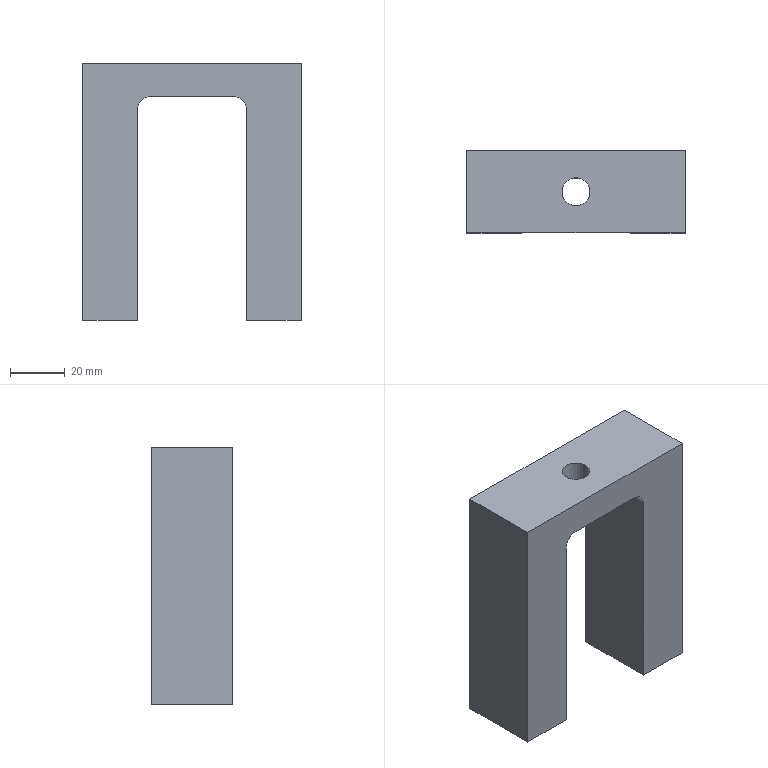Part | STEP file | 11-FG-SJ00211 | 1 solid | 38 faces | box 80 x 30 x 94 mm | volume 125576 mm3 | cylinder 16 | cone 12 | plane 10 | commonest cylinder face diameters 3.3 x8 5 x4 10 x2 10.2 x2
STEP:
#1=CARTESIAN_POINT('',(29.9,9.,70.65));
#2=VERTEX_POINT('',#1);
#3=CARTESIAN_POINT('',(29.9,9.,67.35));
#4=VERTEX_POINT('',#3);
#5=CARTESIAN_POINT('',(29.9,9.,69.));
#6=DIRECTION('',(1.,0.,0.));
#7=DIRECTION('',(0.,0.,-1.));
#8=AXIS2_PLACEMENT_3D('',#5,#6,#7);
#9=CIRCLE('',#8,1.65);
#10=EDGE_CURVE('',#2,#4,#9,.T.);
#11=ORIENTED_EDGE('',*,*,#10,.F.);
#12=CARTESIAN_POINT('',(40.,9.,70.65));
#13=VERTEX_POINT('',#12);
#14=CARTESIAN_POINT('',(40.,9.,70.65));
#15=DIRECTION('',(1.,0.,0.));
#16=VECTOR('',#15,1000.);
#17=LINE('',#14,#16);
#18=EDGE_CURVE('',#2,#13,#17,.T.);
#19=ORIENTED_EDGE('',*,*,#18,.T.);
#20=CARTESIAN_POINT('',(40.,9.,67.35));
#21=VERTEX_POINT('',#20);
#22=CARTESIAN_POINT('',(40.,9.,69.));
#23=DIRECTION('',(1.,0.,0.));
#24=DIRECTION('',(0.,0.,-1.));
#25=AXIS2_PLACEMENT_3D('',#22,#23,#24);
#26=CIRCLE('',#25,1.65);
#27=EDGE_CURVE('',#13,#21,#26,.T.);
#28=ORIENTED_EDGE('',*,*,#27,.T.);
#29=CARTESIAN_POINT('',(40.,9.,67.35));
#30=DIRECTION('',(1.,0.,0.));
#31=VECTOR('',#30,1000.);
#32=LINE('',#29,#31);
#33=EDGE_CURVE('',#4,#21,#32,.T.);
#34=ORIENTED_EDGE('',*,*,#33,.F.);
#35=EDGE_LOOP('',(#11,#19,#28,#34));
#36=FACE_OUTER_BOUND('',#35,.T.);
#37=CARTESIAN_POINT('',(40.,9.,69.));
#38=DIRECTION('',(1.,0.,0.));
#39=DIRECTION('',(0.,0.,-1.));
#40=AXIS2_PLACEMENT_3D('',#37,#38,#39);
#41=CYLINDRICAL_SURFACE('',#40,1.65);
#42=ADVANCED_FACE('',(#36),#41,.F.);
#43=CARTESIAN_POINT('',(28.909,9.,69.));
#44=VERTEX_POINT('',#43);
#45=CARTESIAN_POINT('',(29.9,9.,67.35));
#46=DIRECTION('',(0.515,0.,-0.8572));
#47=VECTOR('',#46,1000.);
#48=LINE('',#45,#47);
#49=EDGE_CURVE('',#44,#4,#48,.T.);
#50=ORIENTED_EDGE('',*,*,#49,.F.);
#51=CARTESIAN_POINT('',(29.9,9.,70.65));
#52=DIRECTION('',(0.515,0.,0.8572));
#53=VECTOR('',#52,1000.);
#54=LINE('',#51,#53);
#55=EDGE_CURVE('',#44,#2,#54,.T.);
#56=ORIENTED_EDGE('',*,*,#55,.T.);
#57=ORIENTED_EDGE('',*,*,#10,.T.);
#58=EDGE_LOOP('',(#50,#56,#57));
#59=FACE_OUTER_BOUND('',#58,.T.);
#60=CARTESIAN_POINT('',(29.9,9.,69.));
#61=DIRECTION('',(1.,0.,0.));
#62=DIRECTION('',(0.,0.,-1.));
#63=AXIS2_PLACEMENT_3D('',#60,#61,#62);
#64=CONICAL_SURFACE('',#63,1.65,1.03);
#65=ADVANCED_FACE('',(#59),#64,.F.);
#66=CARTESIAN_POINT('',(29.9,9.,86.65));
#67=VERTEX_POINT('',#66);
#68=CARTESIAN_POINT('',(29.9,9.,83.35));
#69=VERTEX_POINT('',#68);
#70=CARTESIAN_POINT('',(29.9,9.,85.));
#71=DIRECTION('',(1.,0.,0.));
#72=DIRECTION('',(0.,0.,-1.));
#73=AXIS2_PLACEMENT_3D('',#70,#71,#72);
#74=CIRCLE('',#73,1.65);
#75=EDGE_CURVE('',#67,#69,#74,.T.);
#76=ORIENTED_EDGE('',*,*,#75,.F.);
#77=CARTESIAN_POINT('',(40.,9.,86.65));
#78=VERTEX_POINT('',#77);
#79=CARTESIAN_POINT('',(40.,9.,86.65));
#80=DIRECTION('',(1.,0.,0.));
#81=VECTOR('',#80,1000.);
#82=LINE('',#79,#81);
#83=EDGE_CURVE('',#67,#78,#82,.T.);
#84=ORIENTED_EDGE('',*,*,#83,.T.);
#85=CARTESIAN_POINT('',(40.,9.,83.35));
#86=VERTEX_POINT('',#85);
#87=CARTESIAN_POINT('',(40.,9.,85.));
#88=DIRECTION('',(1.,0.,0.));
#89=DIRECTION('',(0.,0.,-1.));
#90=AXIS2_PLACEMENT_3D('',#87,#88,#89);
#91=CIRCLE('',#90,1.65);
#92=EDGE_CURVE('',#78,#86,#91,.T.);
#93=ORIENTED_EDGE('',*,*,#92,.T.);
#94=CARTESIAN_POINT('',(40.,9.,83.35));
#95=DIRECTION('',(1.,0.,0.));
#96=VECTOR('',#95,1000.);
#97=LINE('',#94,#96);
#98=EDGE_CURVE('',#69,#86,#97,.T.);
#99=ORIENTED_EDGE('',*,*,#98,.F.);
#100=EDGE_LOOP('',(#76,#84,#93,#99));
#101=FACE_OUTER_BOUND('',#100,.T.);
#102=CARTESIAN_POINT('',(40.,9.,85.));
#103=DIRECTION('',(1.,0.,0.));
#104=DIRECTION('',(0.,0.,-1.));
#105=AXIS2_PLACEMENT_3D('',#102,#103,#104);
#106=CYLINDRICAL_SURFACE('',#105,1.65);
#107=ADVANCED_FACE('',(#101),#106,.F.);
#108=CARTESIAN_POINT('',(28.909,9.,85.));
#109=VERTEX_POINT('',#108);
#110=CARTESIAN_POINT('',(29.9,9.,83.35));
#111=DIRECTION('',(0.515,0.,-0.8572));
#112=VECTOR('',#111,1000.);
#113=LINE('',#110,#112);
#114=EDGE_CURVE('',#109,#69,#113,.T.);
#115=ORIENTED_EDGE('',*,*,#114,.F.);
#116=CARTESIAN_POINT('',(29.9,9.,86.65));
#117=DIRECTION('',(0.515,0.,0.8572));
#118=VECTOR('',#117,1000.);
#119=LINE('',#116,#118);
#120=EDGE_CURVE('',#109,#67,#119,.T.);
#121=ORIENTED_EDGE('',*,*,#120,.T.);
#122=ORIENTED_EDGE('',*,*,#75,.T.);
#123=EDGE_LOOP('',(#115,#121,#122));
#124=FACE_OUTER_BOUND('',#123,.T.);
#125=CARTESIAN_POINT('',(29.9,9.,85.));
#126=DIRECTION('',(1.,0.,0.));
#127=DIRECTION('',(0.,0.,-1.));
#128=AXIS2_PLACEMENT_3D('',#125,#126,#127);
#129=CONICAL_SURFACE('',#128,1.65,1.03);
#130=ADVANCED_FACE('',(#124),#129,.F.);
#131=CARTESIAN_POINT('',(29.9,-9.,86.65));
#132=VERTEX_POINT('',#131);
#133=CARTESIAN_POINT('',(29.9,-9.,83.35));
#134=VERTEX_POINT('',#133);
#135=CARTESIAN_POINT('',(29.9,-9.,85.));
#136=DIRECTION('',(1.,0.,0.));
#137=DIRECTION('',(0.,0.,-1.));
#138=AXIS2_PLACEMENT_3D('',#135,#136,#137);
#139=CIRCLE('',#138,1.65);
#140=EDGE_CURVE('',#132,#134,#139,.T.);
#141=ORIENTED_EDGE('',*,*,#140,.F.);
#142=CARTESIAN_POINT('',(40.,-9.,86.65));
#143=VERTEX_POINT('',#142);
#144=CARTESIAN_POINT('',(40.,-9.,86.65));
#145=DIRECTION('',(1.,0.,0.));
#146=VECTOR('',#145,1000.);
#147=LINE('',#144,#146);
#148=EDGE_CURVE('',#132,#143,#147,.T.);
#149=ORIENTED_EDGE('',*,*,#148,.T.);
#150=CARTESIAN_POINT('',(40.,-9.,83.35));
#151=VERTEX_POINT('',#150);
#152=CARTESIAN_POINT('',(40.,-9.,85.));
#153=DIRECTION('',(1.,0.,0.));
#154=DIRECTION('',(0.,0.,-1.));
#155=AXIS2_PLACEMENT_3D('',#152,#153,#154);
#156=CIRCLE('',#155,1.65);
#157=EDGE_CURVE('',#143,#151,#156,.T.);
#158=ORIENTED_EDGE('',*,*,#157,.T.);
#159=CARTESIAN_POINT('',(40.,-9.,83.35));
#160=DIRECTION('',(1.,0.,0.));
#161=VECTOR('',#160,1000.);
#162=LINE('',#159,#161);
#163=EDGE_CURVE('',#134,#151,#162,.T.);
#164=ORIENTED_EDGE('',*,*,#163,.F.);
#165=EDGE_LOOP('',(#141,#149,#158,#164));
#166=FACE_OUTER_BOUND('',#165,.T.);
#167=CARTESIAN_POINT('',(40.,-9.,85.));
#168=DIRECTION('',(1.,0.,0.));
#169=DIRECTION('',(0.,0.,-1.));
#170=AXIS2_PLACEMENT_3D('',#167,#168,#169);
#171=CYLINDRICAL_SURFACE('',#170,1.65);
#172=ADVANCED_FACE('',(#166),#171,.F.);
#173=CARTESIAN_POINT('',(28.909,-9.,85.));
#174=VERTEX_POINT('',#173);
#175=CARTESIAN_POINT('',(29.9,-9.,83.35));
#176=DIRECTION('',(0.515,0.,-0.8572));
#177=VECTOR('',#176,1000.);
#178=LINE('',#175,#177);
#179=EDGE_CURVE('',#174,#134,#178,.T.);
#180=ORIENTED_EDGE('',*,*,#179,.F.);
#181=CARTESIAN_POINT('',(29.9,-9.,86.65));
#182=DIRECTION('',(0.515,0.,0.8572));
#183=VECTOR('',#182,1000.);
#184=LINE('',#181,#183);
#185=EDGE_CURVE('',#174,#132,#184,.T.);
#186=ORIENTED_EDGE('',*,*,#185,.T.);
#187=ORIENTED_EDGE('',*,*,#140,.T.);
#188=EDGE_LOOP('',(#180,#186,#187));
#189=FACE_OUTER_BOUND('',#188,.T.);
#190=CARTESIAN_POINT('',(29.9,-9.,85.));
#191=DIRECTION('',(1.,0.,0.));
#192=DIRECTION('',(0.,0.,-1.));
#193=AXIS2_PLACEMENT_3D('',#190,#191,#192);
#194=CONICAL_SURFACE('',#193,1.65,1.03);
#195=ADVANCED_FACE('',(#189),#194,.F.);
#196=CARTESIAN_POINT('',(29.9,-9.,70.65));
#197=VERTEX_POINT('',#196);
#198=CARTESIAN_POINT('',(29.9,-9.,67.35));
#199=VERTEX_POINT('',#198);
#200=CARTESIAN_POINT('',(29.9,-9.,69.));
#201=DIRECTION('',(1.,0.,0.));
#202=DIRECTION('',(0.,0.,-1.));
#203=AXIS2_PLACEMENT_3D('',#200,#201,#202);
#204=CIRCLE('',#203,1.65);
#205=EDGE_CURVE('',#197,#199,#204,.T.);
#206=ORIENTED_EDGE('',*,*,#205,.F.);
#207=CARTESIAN_POINT('',(40.,-9.,70.65));
#208=VERTEX_POINT('',#207);
#209=CARTESIAN_POINT('',(40.,-9.,70.65));
#210=DIRECTION('',(1.,0.,0.));
#211=VECTOR('',#210,1000.);
#212=LINE('',#209,#211);
#213=EDGE_CURVE('',#197,#208,#212,.T.);
#214=ORIENTED_EDGE('',*,*,#213,.T.);
#215=CARTESIAN_POINT('',(40.,-9.,67.35));
#216=VERTEX_POINT('',#215);
#217=CARTESIAN_POINT('',(40.,-9.,69.));
#218=DIRECTION('',(1.,0.,0.));
#219=DIRECTION('',(0.,0.,-1.));
#220=AXIS2_PLACEMENT_3D('',#217,#218,#219);
#221=CIRCLE('',#220,1.65);
#222=EDGE_CURVE('',#208,#216,#221,.T.);
#223=ORIENTED_EDGE('',*,*,#222,.T.);
#224=CARTESIAN_POINT('',(40.,-9.,67.35));
#225=DIRECTION('',(1.,0.,0.));
#226=VECTOR('',#225,1000.);
#227=LINE('',#224,#226);
#228=EDGE_CURVE('',#199,#216,#227,.T.);
#229=ORIENTED_EDGE('',*,*,#228,.F.);
#230=EDGE_LOOP('',(#206,#214,#223,#229));
#231=FACE_OUTER_BOUND('',#230,.T.);
#232=CARTESIAN_POINT('',(40.,-9.,69.));
#233=DIRECTION('',(1.,0.,0.));
#234=DIRECTION('',(0.,0.,-1.));
#235=AXIS2_PLACEMENT_3D('',#232,#233,#234);
#236=CYLINDRICAL_SURFACE('',#235,1.65);
#237=ADVANCED_FACE('',(#231),#236,.F.);
#238=CARTESIAN_POINT('',(28.909,-9.,69.));
#239=VERTEX_POINT('',#238);
#240=CARTESIAN_POINT('',(29.9,-9.,67.35));
#241=DIRECTION('',(0.515,0.,-0.8572));
#242=VECTOR('',#241,1000.);
#243=LINE('',#240,#242);
#244=EDGE_CURVE('',#239,#199,#243,.T.);
#245=ORIENTED_EDGE('',*,*,#244,.F.);
#246=CARTESIAN_POINT('',(29.9,-9.,70.65));
#247=DIRECTION('',(0.515,0.,0.8572));
#248=VECTOR('',#247,1000.);
#249=LINE('',#246,#248);
#250=EDGE_CURVE('',#239,#197,#249,.T.);
#251=ORIENTED_EDGE('',*,*,#250,.T.);
#252=ORIENTED_EDGE('',*,*,#205,.T.);
#253=EDGE_LOOP('',(#245,#251,#252));
#254=FACE_OUTER_BOUND('',#253,.T.);
#255=CARTESIAN_POINT('',(29.9,-9.,69.));
#256=DIRECTION('',(1.,0.,0.));
#257=DIRECTION('',(0.,0.,-1.));
#258=AXIS2_PLACEMENT_3D('',#255,#256,#257);
#259=CONICAL_SURFACE('',#258,1.65,1.03);
#260=ADVANCED_FACE('',(#254),#259,.F.);
#261=CARTESIAN_POINT('',(-27.5,0.,15.));
#262=VERTEX_POINT('',#261);
#263=CARTESIAN_POINT('',(-32.5,0.,15.));
#264=VERTEX_POINT('',#263);
#265=CARTESIAN_POINT('',(-30.,0.,15.));
#266=DIRECTION('',(0.,0.,-1.));
#267=DIRECTION('',(-1.,0.,0.));
#268=AXIS2_PLACEMENT_3D('',#265,#266,#267);
#269=CIRCLE('',#268,2.5);
#270=EDGE_CURVE('',#262,#264,#269,.T.);
#271=ORIENTED_EDGE('',*,*,#270,.F.);
#272=CARTESIAN_POINT('',(-27.5,0.,0.));
#273=VERTEX_POINT('',#272);
#274=CARTESIAN_POINT('',(-27.5,0.,0.));
#275=DIRECTION('',(0.,0.,-1.));
#276=VECTOR('',#275,1000.);
#277=LINE('',#274,#276);
#278=EDGE_CURVE('',#262,#273,#277,.T.);
#279=ORIENTED_EDGE('',*,*,#278,.T.);
#280=CARTESIAN_POINT('',(-32.5,0.,0.));
#281=VERTEX_POINT('',#280);
#282=CARTESIAN_POINT('',(-30.,0.,0.));
#283=DIRECTION('',(0.,0.,-1.));
#284=DIRECTION('',(-1.,0.,0.));
#285=AXIS2_PLACEMENT_3D('',#282,#283,#284);
#286=CIRCLE('',#285,2.5);
#287=EDGE_CURVE('',#273,#281,#286,.T.);
#288=ORIENTED_EDGE('',*,*,#287,.T.);
#289=CARTESIAN_POINT('',(-32.5,0.,0.));
#290=DIRECTION('',(0.,0.,-1.));
#291=VECTOR('',#290,1000.);
#292=LINE('',#289,#291);
#293=EDGE_CURVE('',#264,#281,#292,.T.);
#294=ORIENTED_EDGE('',*,*,#293,.F.);
#295=EDGE_LOOP('',(#271,#279,#288,#294));
#296=FACE_OUTER_BOUND('',#295,.T.);
#297=CARTESIAN_POINT('',(-30.,0.,0.));
#298=DIRECTION('',(0.,0.,-1.));
#299=DIRECTION('',(-1.,0.,0.));
#300=AXIS2_PLACEMENT_3D('',#297,#298,#299);
#301=CYLINDRICAL_SURFACE('',#300,2.5);
#302=ADVANCED_FACE('',(#296),#301,.F.);
#303=CARTESIAN_POINT('',(-30.,0.,16.502));
#304=VERTEX_POINT('',#303);
#305=CARTESIAN_POINT('',(-32.5,0.,15.));
#306=DIRECTION('',(-0.8572,0.,-0.515));
#307=VECTOR('',#306,1000.);
#308=LINE('',#305,#307);
#309=EDGE_CURVE('',#304,#264,#308,.T.);
#310=ORIENTED_EDGE('',*,*,#309,.F.);
#311=CARTESIAN_POINT('',(-27.5,0.,15.));
#312=DIRECTION('',(0.8572,0.,-0.515));
#313=VECTOR('',#312,1000.);
#314=LINE('',#311,#313);
#315=EDGE_CURVE('',#304,#262,#314,.T.);
#316=ORIENTED_EDGE('',*,*,#315,.T.);
#317=ORIENTED_EDGE('',*,*,#270,.T.);
#318=EDGE_LOOP('',(#310,#316,#317));
#319=FACE_OUTER_BOUND('',#318,.T.);
#320=CARTESIAN_POINT('',(-30.,0.,15.));
#321=DIRECTION('',(0.,0.,-1.));
#322=DIRECTION('',(-1.,0.,0.));
#323=AXIS2_PLACEMENT_3D('',#320,#321,#322);
#324=CONICAL_SURFACE('',#323,2.5,1.03);
#325=ADVANCED_FACE('',(#319),#324,.F.);
#326=CARTESIAN_POINT('',(32.5,0.,15.));
#327=VERTEX_POINT('',#326);
#328=CARTESIAN_POINT('',(27.5,0.,15.));
#329=VERTEX_POINT('',#328);
#330=CARTESIAN_POINT('',(30.,0.,15.));
#331=DIRECTION('',(0.,0.,-1.));
#332=DIRECTION('',(-1.,0.,0.));
#333=AXIS2_PLACEMENT_3D('',#330,#331,#332);
#334=CIRCLE('',#333,2.5);
#335=EDGE_CURVE('',#327,#329,#334,.T.);
#336=ORIENTED_EDGE('',*,*,#335,.F.);
#337=CARTESIAN_POINT('',(32.5,0.,0.));
#338=VERTEX_POINT('',#337);
#339=CARTESIAN_POINT('',(32.5,0.,0.));
#340=DIRECTION('',(0.,0.,-1.));
#341=VECTOR('',#340,1000.);
#342=LINE('',#339,#341);
#343=EDGE_CURVE('',#327,#338,#342,.T.);
#344=ORIENTED_EDGE('',*,*,#343,.T.);
#345=CARTESIAN_POINT('',(27.5,0.,0.));
#346=VERTEX_POINT('',#345);
#347=CARTESIAN_POINT('',(30.,0.,0.));
#348=DIRECTION('',(0.,0.,-1.));
#349=DIRECTION('',(-1.,0.,0.));
#350=AXIS2_PLACEMENT_3D('',#347,#348,#349);
#351=CIRCLE('',#350,2.5);
#352=EDGE_CURVE('',#338,#346,#351,.T.);
#353=ORIENTED_EDGE('',*,*,#352,.T.);
#354=CARTESIAN_POINT('',(27.5,0.,0.));
#355=DIRECTION('',(0.,0.,-1.));
#356=VECTOR('',#355,1000.);
#357=LINE('',#354,#356);
#358=EDGE_CURVE('',#329,#346,#357,.T.);
#359=ORIENTED_EDGE('',*,*,#358,.F.);
#360=EDGE_LOOP('',(#336,#344,#353,#359));
#361=FACE_OUTER_BOUND('',#360,.T.);
#362=CARTESIAN_POINT('',(30.,0.,0.));
#363=DIRECTION('',(0.,0.,-1.));
#364=DIRECTION('',(-1.,0.,0.));
#365=AXIS2_PLACEMENT_3D('',#362,#363,#364);
#366=CYLINDRICAL_SURFACE('',#365,2.5);
#367=ADVANCED_FACE('',(#361),#366,.F.);
#368=CARTESIAN_POINT('',(30.,0.,16.502));
#369=VERTEX_POINT('',#368);
#370=CARTESIAN_POINT('',(27.5,0.,15.));
#371=DIRECTION('',(-0.8572,0.,-0.515));
#372=VECTOR('',#371,1000.);
#373=LINE('',#370,#372);
#374=EDGE_CURVE('',#369,#329,#373,.T.);
#375=ORIENTED_EDGE('',*,*,#374,.F.);
#376=CARTESIAN_POINT('',(32.5,0.,15.));
#377=DIRECTION('',(0.8572,0.,-0.515));
#378=VECTOR('',#377,1000.);
#379=LINE('',#376,#378);
#380=EDGE_CURVE('',#369,#327,#379,.T.);
#381=ORIENTED_EDGE('',*,*,#380,.T.);
#382=ORIENTED_EDGE('',*,*,#335,.T.);
#383=EDGE_LOOP('',(#375,#381,#382));
#384=FACE_OUTER_BOUND('',#383,.T.);
#385=CARTESIAN_POINT('',(30.,0.,15.));
#386=DIRECTION('',(0.,0.,-1.));
#387=DIRECTION('',(-1.,0.,0.));
#388=AXIS2_PLACEMENT_3D('',#385,#386,#387);
#389=CONICAL_SURFACE('',#388,2.5,1.03);
#390=ADVANCED_FACE('',(#384),#389,.F.);
#391=CARTESIAN_POINT('',(-5.1,0.,82.));
#392=VERTEX_POINT('',#391);
#393=CARTESIAN_POINT('',(5.1,0.,82.));
#394=VERTEX_POINT('',#393);
#395=CARTESIAN_POINT('',(0.,0.,82.));
#396=DIRECTION('',(0.,0.,1.));
#397=DIRECTION('',(1.,0.,0.));
#398=AXIS2_PLACEMENT_3D('',#395,#396,#397);
#399=CIRCLE('',#398,5.1);
#400=EDGE_CURVE('',#392,#394,#399,.T.);
#401=ORIENTED_EDGE('',*,*,#400,.F.);
#402=CARTESIAN_POINT('',(-5.1,0.,94.));
#403=VERTEX_POINT('',#402);
#404=CARTESIAN_POINT('',(-5.1,0.,94.));
#405=DIRECTION('',(0.,0.,1.));
#406=VECTOR('',#405,1000.);
#407=LINE('',#404,#406);
#408=EDGE_CURVE('',#392,#403,#407,.T.);
#409=ORIENTED_EDGE('',*,*,#408,.T.);
#410=CARTESIAN_POINT('',(5.1,0.,94.));
#411=VERTEX_POINT('',#410);
#412=CARTESIAN_POINT('',(0.,0.,94.));
#413=DIRECTION('',(0.,0.,1.));
#414=DIRECTION('',(1.,0.,0.));
#415=AXIS2_PLACEMENT_3D('',#412,#413,#414);
#416=CIRCLE('',#415,5.1);
#417=EDGE_CURVE('',#403,#411,#416,.T.);
#418=ORIENTED_EDGE('',*,*,#417,.T.);
#419=CARTESIAN_POINT('',(5.1,0.,94.));
#420=DIRECTION('',(0.,0.,1.));
#421=VECTOR('',#420,1000.);
#422=LINE('',#419,#421);
#423=EDGE_CURVE('',#394,#411,#422,.T.);
#424=ORIENTED_EDGE('',*,*,#423,.F.);
#425=EDGE_LOOP('',(#401,#409,#418,#424));
#426=FACE_OUTER_BOUND('',#425,.T.);
#427=CARTESIAN_POINT('',(0.,0.,94.));
#428=DIRECTION('',(0.,0.,1.));
#429=DIRECTION('',(1.,0.,0.));
#430=AXIS2_PLACEMENT_3D('',#427,#428,#429);
#431=CYLINDRICAL_SURFACE('',#430,5.1);
#432=ADVANCED_FACE('',(#426),#431,.F.);
#433=CARTESIAN_POINT('',(30.,0.,0.));
#434=DIRECTION('',(0.,0.,-1.));
#435=DIRECTION('',(-1.,0.,0.));
#436=AXIS2_PLACEMENT_3D('',#433,#434,#435);
#437=CIRCLE('',#436,2.5);
#438=EDGE_CURVE('',#346,#338,#437,.T.);
#439=ORIENTED_EDGE('',*,*,#438,.F.);
#440=ORIENTED_EDGE('',*,*,#352,.F.);
#441=EDGE_LOOP('',(#439,#440));
#442=FACE_BOUND('',#441,.T.);
#443=CARTESIAN_POINT('',(20.,-15.,0.));
#444=VERTEX_POINT('',#443);
#445=CARTESIAN_POINT('',(40.,-15.,0.));
#446=VERTEX_POINT('',#445);
#447=CARTESIAN_POINT('',(40.,-15.,0.));
#448=DIRECTION('',(1.,0.,0.));
#449=VECTOR('',#448,1000.);
#450=LINE('',#447,#449);
#451=EDGE_CURVE('',#444,#446,#450,.T.);
#452=ORIENTED_EDGE('',*,*,#451,.F.);
#453=CARTESIAN_POINT('',(20.,15.,0.));
#454=VERTEX_POINT('',#453);
#455=CARTESIAN_POINT('',(20.,0.,0.));
#456=DIRECTION('',(0.,1.,0.));
#457=VECTOR('',#456,1000.);
#458=LINE('',#455,#457);
#459=EDGE_CURVE('',#444,#454,#458,.T.);
#460=ORIENTED_EDGE('',*,*,#459,.T.);
#461=CARTESIAN_POINT('',(40.,15.,0.));
#462=VERTEX_POINT('',#461);
#463=CARTESIAN_POINT('',(40.,15.,0.));
#464=DIRECTION('',(-1.,0.,0.));
#465=VECTOR('',#464,1000.);
#466=LINE('',#463,#465);
#467=EDGE_CURVE('',#462,#454,#466,.T.);
#468=ORIENTED_EDGE('',*,*,#467,.F.);
#469=CARTESIAN_POINT('',(40.,-15.,0.));
#470=DIRECTION('',(0.,1.,0.));
#471=VECTOR('',#470,1000.);
#472=LINE('',#469,#471);
#473=EDGE_CURVE('',#446,#462,#472,.T.);
#474=ORIENTED_EDGE('',*,*,#473,.F.);
#475=EDGE_LOOP('',(#452,#460,#468,#474));
#476=FACE_OUTER_BOUND('',#475,.T.);
#477=CARTESIAN_POINT('',(0.,0.,0.));
#478=DIRECTION('',(0.,0.,1.));
#479=DIRECTION('',(1.,0.,0.));
#480=AXIS2_PLACEMENT_3D('',#477,#478,#479);
#481=PLANE('',#480);
#482=ADVANCED_FACE('',(#442,#476),#481,.F.);
#483=CARTESIAN_POINT('',(-40.,15.,0.));
#484=VERTEX_POINT('',#483);
#485=CARTESIAN_POINT('',(-40.,-15.,0.));
#486=VERTEX_POINT('',#485);
#487=CARTESIAN_POINT('',(-40.,-15.,0.));
#488=DIRECTION('',(0.,-1.,0.));
#489=VECTOR('',#488,1000.);
#490=LINE('',#487,#489);
#491=EDGE_CURVE('',#484,#486,#490,.T.);
#492=ORIENTED_EDGE('',*,*,#491,.T.);
#493=CARTESIAN_POINT('',(-40.,-15.,94.));
#494=VERTEX_POINT('',#493);
#495=CARTESIAN_POINT('',(-40.,-15.,94.));
#496=DIRECTION('',(0.,0.,-1.));
#497=VECTOR('',#496,1000.);
#498=LINE('',#495,#497);
#499=EDGE_CURVE('',#494,#486,#498,.T.);
#500=ORIENTED_EDGE('',*,*,#499,.F.);
#501=CARTESIAN_POINT('',(-40.,15.,94.));
#502=VERTEX_POINT('',#501);
#503=CARTESIAN_POINT('',(-40.,-15.,94.));
#504=DIRECTION('',(0.,-1.,0.));
#505=VECTOR('',#504,1000.);
#506=LINE('',#503,#505);
#507=EDGE_CURVE('',#502,#494,#506,.T.);
#508=ORIENTED_EDGE('',*,*,#507,.F.);
#509=CARTESIAN_POINT('',(-40.,15.,94.));
#510=DIRECTION('',(0.,0.,-1.));
#511=VECTOR('',#510,1000.);
#512=LINE('',#509,#511);
#513=EDGE_CURVE('',#502,#484,#512,.T.);
#514=ORIENTED_EDGE('',*,*,#513,.T.);
#515=EDGE_LOOP('',(#492,#500,#508,#514));
#516=FACE_OUTER_BOUND('',#515,.T.);
#517=CARTESIAN_POINT('',(-40.,-15.,94.));
#518=DIRECTION('',(1.,0.,0.));
#519=DIRECTION('',(0.,0.,-1.));
#520=AXIS2_PLACEMENT_3D('',#517,#518,#519);
#521=PLANE('',#520);
#522=ADVANCED_FACE('',(#516),#521,.F.);
#523=CARTESIAN_POINT('',(20.,-15.,77.));
#524=VERTEX_POINT('',#523);
#525=CARTESIAN_POINT('',(15.,-15.,82.));
#526=VERTEX_POINT('',#525);
#527=CARTESIAN_POINT('',(15.,-15.,77.));
#528=DIRECTION('',(0.,-1.,0.));
#529=DIRECTION('',(1.,0.,0.));
#530=AXIS2_PLACEMENT_3D('',#527,#528,#529);
#531=CIRCLE('',#530,5.);
#532=EDGE_CURVE('',#524,#526,#531,.T.);
#533=ORIENTED_EDGE('',*,*,#532,.F.);
#534=CARTESIAN_POINT('',(20.,-15.,-82.));
#535=DIRECTION('',(0.,0.,1.));
#536=VECTOR('',#535,1000.);
#537=LINE('',#534,#536);
#538=EDGE_CURVE('',#444,#524,#537,.T.);
#539=ORIENTED_EDGE('',*,*,#538,.F.);
#540=ORIENTED_EDGE('',*,*,#451,.T.);
#541=CARTESIAN_POINT('',(40.,-15.,94.));
#542=VERTEX_POINT('',#541);
#543=CARTESIAN_POINT('',(40.,-15.,94.));
#544=DIRECTION('',(0.,0.,-1.));
#545=VECTOR('',#544,1000.);
#546=LINE('',#543,#545);
#547=EDGE_CURVE('',#542,#446,#546,.T.);
#548=ORIENTED_EDGE('',*,*,#547,.F.);
#549=CARTESIAN_POINT('',(40.,-15.,94.));
#550=DIRECTION('',(1.,0.,0.));
#551=VECTOR('',#550,1000.);
#552=LINE('',#549,#551);
#553=EDGE_CURVE('',#494,#542,#552,.T.);
#554=ORIENTED_EDGE('',*,*,#553,.F.);
#555=ORIENTED_EDGE('',*,*,#499,.T.);
#556=CARTESIAN_POINT('',(-20.,-15.,0.));
#557=VERTEX_POINT('',#556);
#558=CARTESIAN_POINT('',(40.,-15.,0.));
#559=DIRECTION('',(1.,0.,0.));
#560=VECTOR('',#559,1000.);
#561=LINE('',#558,#560);
#562=EDGE_CURVE('',#486,#557,#561,.T.);
#563=ORIENTED_EDGE('',*,*,#562,.T.);
#564=CARTESIAN_POINT('',(-20.,-15.,77.));
#565=VERTEX_POINT('',#564);
#566=CARTESIAN_POINT('',(-20.,-15.,-82.));
#567=DIRECTION('',(0.,0.,-1.));
#568=VECTOR('',#567,1000.);
#569=LINE('',#566,#568);
#570=EDGE_CURVE('',#565,#557,#569,.T.);
#571=ORIENTED_EDGE('',*,*,#570,.F.);
#572=CARTESIAN_POINT('',(-15.,-15.,82.));
#573=VERTEX_POINT('',#572);
#574=CARTESIAN_POINT('',(-15.,-15.,77.));
#575=DIRECTION('',(0.,-1.,0.));
#576=DIRECTION('',(1.,0.,0.));
#577=AXIS2_PLACEMENT_3D('',#574,#575,#576);
#578=CIRCLE('',#577,5.);
#579=EDGE_CURVE('',#573,#565,#578,.T.);
#580=ORIENTED_EDGE('',*,*,#579,.F.);
#581=CARTESIAN_POINT('',(15.,-15.,82.));
#582=DIRECTION('',(-1.,0.,0.));
#583=VECTOR('',#582,1000.);
#584=LINE('',#581,#583);
#585=EDGE_CURVE('',#526,#573,#584,.T.);
#586=ORIENTED_EDGE('',*,*,#585,.F.);
#587=EDGE_LOOP('',(#533,#539,#540,#548,#554,#555,#563,#571,#580,#586));
#588=FACE_OUTER_BOUND('',#587,.T.);
#589=CARTESIAN_POINT('',(40.,-15.,94.));
#590=DIRECTION('',(0.,1.,0.));
#591=DIRECTION('',(-1.,0.,0.));
#592=AXIS2_PLACEMENT_3D('',#589,#590,#591);
#593=PLANE('',#592);
#594=ADVANCED_FACE('',(#588),#593,.F.);
#595=CARTESIAN_POINT('',(40.,9.,69.));
#596=DIRECTION('',(1.,0.,0.));
#597=DIRECTION('',(0.,0.,-1.));
#598=AXIS2_PLACEMENT_3D('',#595,#596,#597);
#599=CIRCLE('',#598,1.65);
#600=EDGE_CURVE('',#21,#13,#599,.T.);
#601=ORIENTED_EDGE('',*,*,#600,.F.);
#602=ORIENTED_EDGE('',*,*,#27,.F.);
#603=EDGE_LOOP('',(#601,#602));
#604=FACE_BOUND('',#603,.T.);
#605=CARTESIAN_POINT('',(40.,9.,85.));
#606=DIRECTION('',(1.,0.,0.));
#607=DIRECTION('',(0.,0.,-1.));
#608=AXIS2_PLACEMENT_3D('',#605,#606,#607);
#609=CIRCLE('',#608,1.65);
#610=EDGE_CURVE('',#86,#78,#609,.T.);
#611=ORIENTED_EDGE('',*,*,#610,.F.);
#612=ORIENTED_EDGE('',*,*,#92,.F.);
#613=EDGE_LOOP('',(#611,#612));
#614=FACE_BOUND('',#613,.T.);
#615=CARTESIAN_POINT('',(40.,-9.,85.));
#616=DIRECTION('',(1.,0.,0.));
#617=DIRECTION('',(0.,0.,-1.));
#618=AXIS2_PLACEMENT_3D('',#615,#616,#617);
#619=CIRCLE('',#618,1.65);
#620=EDGE_CURVE('',#151,#143,#619,.T.);
#621=ORIENTED_EDGE('',*,*,#620,.F.);
#622=ORIENTED_EDGE('',*,*,#157,.F.);
#623=EDGE_LOOP('',(#621,#622));
#624=FACE_BOUND('',#623,.T.);
#625=CARTESIAN_POINT('',(40.,-9.,69.));
#626=DIRECTION('',(1.,0.,0.));
#627=DIRECTION('',(0.,0.,-1.));
#628=AXIS2_PLACEMENT_3D('',#625,#626,#627);
#629=CIRCLE('',#628,1.65);
#630=EDGE_CURVE('',#216,#208,#629,.T.);
#631=ORIENTED_EDGE('',*,*,#630,.F.);
#632=ORIENTED_EDGE('',*,*,#222,.F.);
#633=EDGE_LOOP('',(#631,#632));
#634=FACE_BOUND('',#633,.T.);
#635=ORIENTED_EDGE('',*,*,#473,.T.);
#636=CARTESIAN_POINT('',(40.,15.,94.));
#637=VERTEX_POINT('',#636);
#638=CARTESIAN_POINT('',(40.,15.,94.));
#639=DIRECTION('',(0.,0.,-1.));
#640=VECTOR('',#639,1000.);
#641=LINE('',#638,#640);
#642=EDGE_CURVE('',#637,#462,#641,.T.);
#643=ORIENTED_EDGE('',*,*,#642,.F.);
#644=CARTESIAN_POINT('',(40.,-15.,94.));
#645=DIRECTION('',(0.,1.,0.));
#646=VECTOR('',#645,1000.);
#647=LINE('',#644,#646);
#648=EDGE_CURVE('',#542,#637,#647,.T.);
#649=ORIENTED_EDGE('',*,*,#648,.F.);
#650=ORIENTED_EDGE('',*,*,#547,.T.);
#651=EDGE_LOOP('',(#635,#643,#649,#650));
#652=FACE_OUTER_BOUND('',#651,.T.);
#653=CARTESIAN_POINT('',(40.,-15.,94.));
#654=DIRECTION('',(-1.,0.,0.));
#655=DIRECTION('',(0.,0.,1.));
#656=AXIS2_PLACEMENT_3D('',#653,#654,#655);
#657=PLANE('',#656);
#658=ADVANCED_FACE('',(#604,#614,#624,#634,#652),#657,.F.);
#659=ORIENTED_EDGE('',*,*,#467,.T.);
#660=CARTESIAN_POINT('',(20.,15.,77.));
#661=VERTEX_POINT('',#660);
#662=CARTESIAN_POINT('',(20.,15.,-82.));
#663=DIRECTION('',(0.,0.,1.));
#664=VECTOR('',#663,1000.);
#665=LINE('',#662,#664);
#666=EDGE_CURVE('',#454,#661,#665,.T.);
#667=ORIENTED_EDGE('',*,*,#666,.T.);
#668=CARTESIAN_POINT('',(15.,15.,82.));
#669=VERTEX_POINT('',#668);
#670=CARTESIAN_POINT('',(15.,15.,77.));
#671=DIRECTION('',(0.,-1.,0.));
#672=DIRECTION('',(1.,0.,0.));
#673=AXIS2_PLACEMENT_3D('',#670,#671,#672);
#674=CIRCLE('',#673,5.);
#675=EDGE_CURVE('',#661,#669,#674,.T.);
#676=ORIENTED_EDGE('',*,*,#675,.T.);
#677=CARTESIAN_POINT('',(-15.,15.,82.));
#678=VERTEX_POINT('',#677);
#679=CARTESIAN_POINT('',(15.,15.,82.));
#680=DIRECTION('',(-1.,0.,0.));
#681=VECTOR('',#680,1000.);
#682=LINE('',#679,#681);
#683=EDGE_CURVE('',#669,#678,#682,.T.);
#684=ORIENTED_EDGE('',*,*,#683,.T.);
#685=CARTESIAN_POINT('',(-20.,15.,77.));
#686=VERTEX_POINT('',#685);
#687=CARTESIAN_POINT('',(-15.,15.,77.));
#688=DIRECTION('',(0.,-1.,0.));
#689=DIRECTION('',(1.,0.,0.));
#690=AXIS2_PLACEMENT_3D('',#687,#688,#689);
#691=CIRCLE('',#690,5.);
#692=EDGE_CURVE('',#678,#686,#691,.T.);
#693=ORIENTED_EDGE('',*,*,#692,.T.);
#694=CARTESIAN_POINT('',(-20.,15.,0.));
#695=VERTEX_POINT('',#694);
#696=CARTESIAN_POINT('',(-20.,15.,-82.));
#697=DIRECTION('',(0.,0.,-1.));
#698=VECTOR('',#697,1000.);
#699=LINE('',#696,#698);
#700=EDGE_CURVE('',#686,#695,#699,.T.);
#701=ORIENTED_EDGE('',*,*,#700,.T.);
#702=CARTESIAN_POINT('',(40.,15.,0.));
#703=DIRECTION('',(-1.,0.,0.));
#704=VECTOR('',#703,1000.);
#705=LINE('',#702,#704);
#706=EDGE_CURVE('',#695,#484,#705,.T.);
#707=ORIENTED_EDGE('',*,*,#706,.T.);
#708=ORIENTED_EDGE('',*,*,#513,.F.);
#709=CARTESIAN_POINT('',(40.,15.,94.));
#710=DIRECTION('',(-1.,0.,0.));
#711=VECTOR('',#710,1000.);
#712=LINE('',#709,#711);
#713=EDGE_CURVE('',#637,#502,#712,.T.);
#714=ORIENTED_EDGE('',*,*,#713,.F.);
#715=ORIENTED_EDGE('',*,*,#642,.T.);
#716=EDGE_LOOP('',(#659,#667,#676,#684,#693,#701,#707,#708,#714,#715));
#717=FACE_OUTER_BOUND('',#716,.T.);
#718=CARTESIAN_POINT('',(40.,15.,94.));
#719=DIRECTION('',(0.,-1.,0.));
#720=DIRECTION('',(1.,0.,0.));
#721=AXIS2_PLACEMENT_3D('',#718,#719,#720);
#722=PLANE('',#721);
#723=ADVANCED_FACE('',(#717),#722,.F.);
#724=CARTESIAN_POINT('',(0.,0.,94.));
#725=DIRECTION('',(0.,0.,1.));
#726=DIRECTION('',(1.,0.,0.));
#727=AXIS2_PLACEMENT_3D('',#724,#725,#726);
#728=CIRCLE('',#727,5.1);
#729=EDGE_CURVE('',#411,#403,#728,.T.);
#730=ORIENTED_EDGE('',*,*,#729,.F.);
#731=ORIENTED_EDGE('',*,*,#417,.F.);
#732=EDGE_LOOP('',(#730,#731));
#733=FACE_BOUND('',#732,.T.);
#734=ORIENTED_EDGE('',*,*,#507,.T.);
#735=ORIENTED_EDGE('',*,*,#553,.T.);
#736=ORIENTED_EDGE('',*,*,#648,.T.);
#737=ORIENTED_EDGE('',*,*,#713,.T.);
#738=EDGE_LOOP('',(#734,#735,#736,#737));
#739=FACE_OUTER_BOUND('',#738,.T.);
#740=CARTESIAN_POINT('',(0.,0.,94.));
#741=DIRECTION('',(0.,0.,1.));
#742=DIRECTION('',(1.,0.,0.));
#743=AXIS2_PLACEMENT_3D('',#740,#741,#742);
#744=PLANE('',#743);
#745=ADVANCED_FACE('',(#733,#739),#744,.T.);
#746=CARTESIAN_POINT('',(-30.,0.,0.));
#747=DIRECTION('',(0.,0.,-1.));
#748=DIRECTION('',(-1.,0.,0.));
#749=AXIS2_PLACEMENT_3D('',#746,#747,#748);
#750=CIRCLE('',#749,2.5);
#751=EDGE_CURVE('',#281,#273,#750,.T.);
#752=ORIENTED_EDGE('',*,*,#751,.F.);
#753=ORIENTED_EDGE('',*,*,#287,.F.);
#754=EDGE_LOOP('',(#752,#753));
#755=FACE_BOUND('',#754,.T.);
#756=ORIENTED_EDGE('',*,*,#706,.F.);
#757=CARTESIAN_POINT('',(-20.,0.,0.));
#758=DIRECTION('',(0.,-1.,0.));
#759=VECTOR('',#758,1000.);
#760=LINE('',#757,#759);
#761=EDGE_CURVE('',#695,#557,#760,.T.);
#762=ORIENTED_EDGE('',*,*,#761,.T.);
#763=ORIENTED_EDGE('',*,*,#562,.F.);
#764=ORIENTED_EDGE('',*,*,#491,.F.);
#765=EDGE_LOOP('',(#756,#762,#763,#764));
#766=FACE_OUTER_BOUND('',#765,.T.);
#767=CARTESIAN_POINT('',(0.,0.,0.));
#768=DIRECTION('',(0.,0.,1.));
#769=DIRECTION('',(1.,0.,0.));
#770=AXIS2_PLACEMENT_3D('',#767,#768,#769);
#771=PLANE('',#770);
#772=ADVANCED_FACE('',(#755,#766),#771,.F.);
#773=ORIENTED_EDGE('',*,*,#538,.T.);
#774=CARTESIAN_POINT('',(20.,15.,77.));
#775=DIRECTION('',(0.,-1.,0.));
#776=VECTOR('',#775,1000.);
#777=LINE('',#774,#776);
#778=EDGE_CURVE('',#661,#524,#777,.T.);
#779=ORIENTED_EDGE('',*,*,#778,.F.);
#780=ORIENTED_EDGE('',*,*,#666,.F.);
#781=ORIENTED_EDGE('',*,*,#459,.F.);
#782=EDGE_LOOP('',(#773,#779,#780,#781));
#783=FACE_OUTER_BOUND('',#782,.T.);
#784=CARTESIAN_POINT('',(20.,15.,-82.));
#785=DIRECTION('',(1.,0.,0.));
#786=DIRECTION('',(0.,1.,0.));
#787=AXIS2_PLACEMENT_3D('',#784,#785,#786);
#788=PLANE('',#787);
#789=ADVANCED_FACE('',(#783),#788,.F.);
#790=ORIENTED_EDGE('',*,*,#700,.F.);
#791=CARTESIAN_POINT('',(-20.,15.,77.));
#792=DIRECTION('',(0.,-1.,0.));
#793=VECTOR('',#792,1000.);
#794=LINE('',#791,#793);
#795=EDGE_CURVE('',#686,#565,#794,.T.);
#796=ORIENTED_EDGE('',*,*,#795,.T.);
#797=ORIENTED_EDGE('',*,*,#570,.T.);
#798=ORIENTED_EDGE('',*,*,#761,.F.);
#799=EDGE_LOOP('',(#790,#796,#797,#798));
#800=FACE_OUTER_BOUND('',#799,.T.);
#801=CARTESIAN_POINT('',(-20.,15.,-82.));
#802=DIRECTION('',(-1.,0.,0.));
#803=DIRECTION('',(0.,-1.,0.));
#804=AXIS2_PLACEMENT_3D('',#801,#802,#803);
#805=PLANE('',#804);
#806=ADVANCED_FACE('',(#800),#805,.F.);
#807=ORIENTED_EDGE('',*,*,#579,.T.);
#808=ORIENTED_EDGE('',*,*,#795,.F.);
#809=ORIENTED_EDGE('',*,*,#692,.F.);
#810=CARTESIAN_POINT('',(-15.,15.,82.));
#811=DIRECTION('',(0.,-1.,0.));
#812=VECTOR('',#811,1000.);
#813=LINE('',#810,#812);
#814=EDGE_CURVE('',#678,#573,#813,.T.);
#815=ORIENTED_EDGE('',*,*,#814,.T.);
#816=EDGE_LOOP('',(#807,#808,#809,#815));
#817=FACE_OUTER_BOUND('',#816,.T.);
#818=CARTESIAN_POINT('',(-15.,15.,77.));
#819=DIRECTION('',(0.,-1.,0.));
#820=DIRECTION('',(1.,0.,0.));
#821=AXIS2_PLACEMENT_3D('',#818,#819,#820);
#822=CYLINDRICAL_SURFACE('',#821,5.);
#823=ADVANCED_FACE('',(#817),#822,.F.);
#824=CARTESIAN_POINT('',(0.,0.,82.));
#825=DIRECTION('',(0.,0.,1.));
#826=DIRECTION('',(1.,0.,0.));
#827=AXIS2_PLACEMENT_3D('',#824,#825,#826);
#828=CIRCLE('',#827,5.1);
#829=EDGE_CURVE('',#394,#392,#828,.T.);
#830=ORIENTED_EDGE('',*,*,#829,.T.);
#831=ORIENTED_EDGE('',*,*,#400,.T.);
#832=EDGE_LOOP('',(#830,#831));
#833=FACE_BOUND('',#832,.T.);
#834=ORIENTED_EDGE('',*,*,#585,.T.);
#835=ORIENTED_EDGE('',*,*,#814,.F.);
#836=ORIENTED_EDGE('',*,*,#683,.F.);
#837=CARTESIAN_POINT('',(15.,15.,82.));
#838=DIRECTION('',(0.,-1.,0.));
#839=VECTOR('',#838,1000.);
#840=LINE('',#837,#839);
#841=EDGE_CURVE('',#669,#526,#840,.T.);
#842=ORIENTED_EDGE('',*,*,#841,.T.);
#843=EDGE_LOOP('',(#834,#835,#836,#842));
#844=FACE_OUTER_BOUND('',#843,.T.);
#845=CARTESIAN_POINT('',(15.,15.,82.));
#846=DIRECTION('',(0.,0.,1.));
#847=DIRECTION('',(1.,0.,0.));
#848=AXIS2_PLACEMENT_3D('',#845,#846,#847);
#849=PLANE('',#848);
#850=ADVANCED_FACE('',(#833,#844),#849,.F.);
#851=ORIENTED_EDGE('',*,*,#532,.T.);
#852=ORIENTED_EDGE('',*,*,#841,.F.);
#853=ORIENTED_EDGE('',*,*,#675,.F.);
#854=ORIENTED_EDGE('',*,*,#778,.T.);
#855=EDGE_LOOP('',(#851,#852,#853,#854));
#856=FACE_OUTER_BOUND('',#855,.T.);
#857=CARTESIAN_POINT('',(15.,15.,77.));
#858=DIRECTION('',(0.,-1.,0.));
#859=DIRECTION('',(1.,0.,0.));
#860=AXIS2_PLACEMENT_3D('',#857,#858,#859);
#861=CYLINDRICAL_SURFACE('',#860,5.);
#862=ADVANCED_FACE('',(#856),#861,.F.);
#863=ORIENTED_EDGE('',*,*,#408,.F.);
#864=ORIENTED_EDGE('',*,*,#829,.F.);
#865=ORIENTED_EDGE('',*,*,#423,.T.);
#866=ORIENTED_EDGE('',*,*,#729,.T.);
#867=EDGE_LOOP('',(#863,#864,#865,#866));
#868=FACE_OUTER_BOUND('',#867,.T.);
#869=CARTESIAN_POINT('',(0.,0.,94.));
#870=DIRECTION('',(0.,0.,1.));
#871=DIRECTION('',(1.,0.,0.));
#872=AXIS2_PLACEMENT_3D('',#869,#870,#871);
#873=CYLINDRICAL_SURFACE('',#872,5.1);
#874=ADVANCED_FACE('',(#868),#873,.F.);
#875=ORIENTED_EDGE('',*,*,#380,.F.);
#876=ORIENTED_EDGE('',*,*,#374,.T.);
#877=CARTESIAN_POINT('',(30.,0.,15.));
#878=DIRECTION('',(0.,0.,-1.));
#879=DIRECTION('',(-1.,0.,0.));
#880=AXIS2_PLACEMENT_3D('',#877,#878,#879);
#881=CIRCLE('',#880,2.5);
#882=EDGE_CURVE('',#329,#327,#881,.T.);
#883=ORIENTED_EDGE('',*,*,#882,.T.);
#884=EDGE_LOOP('',(#875,#876,#883));
#885=FACE_OUTER_BOUND('',#884,.T.);
#886=CARTESIAN_POINT('',(30.,0.,15.));
#887=DIRECTION('',(0.,0.,-1.));
#888=DIRECTION('',(-1.,0.,0.));
#889=AXIS2_PLACEMENT_3D('',#886,#887,#888);
#890=CONICAL_SURFACE('',#889,2.5,1.03);
#891=ADVANCED_FACE('',(#885),#890,.F.);
#892=ORIENTED_EDGE('',*,*,#343,.F.);
#893=ORIENTED_EDGE('',*,*,#882,.F.);
#894=ORIENTED_EDGE('',*,*,#358,.T.);
#895=ORIENTED_EDGE('',*,*,#438,.T.);
#896=EDGE_LOOP('',(#892,#893,#894,#895));
#897=FACE_OUTER_BOUND('',#896,.T.);
#898=CARTESIAN_POINT('',(30.,0.,0.));
#899=DIRECTION('',(0.,0.,-1.));
#900=DIRECTION('',(-1.,0.,0.));
#901=AXIS2_PLACEMENT_3D('',#898,#899,#900);
#902=CYLINDRICAL_SURFACE('',#901,2.5);
#903=ADVANCED_FACE('',(#897),#902,.F.);
#904=ORIENTED_EDGE('',*,*,#315,.F.);
#905=ORIENTED_EDGE('',*,*,#309,.T.);
#906=CARTESIAN_POINT('',(-30.,0.,15.));
#907=DIRECTION('',(0.,0.,-1.));
#908=DIRECTION('',(-1.,0.,0.));
#909=AXIS2_PLACEMENT_3D('',#906,#907,#908);
#910=CIRCLE('',#909,2.5);
#911=EDGE_CURVE('',#264,#262,#910,.T.);
#912=ORIENTED_EDGE('',*,*,#911,.T.);
#913=EDGE_LOOP('',(#904,#905,#912));
#914=FACE_OUTER_BOUND('',#913,.T.);
#915=CARTESIAN_POINT('',(-30.,0.,15.));
#916=DIRECTION('',(0.,0.,-1.));
#917=DIRECTION('',(-1.,0.,0.));
#918=AXIS2_PLACEMENT_3D('',#915,#916,#917);
#919=CONICAL_SURFACE('',#918,2.5,1.03);
#920=ADVANCED_FACE('',(#914),#919,.F.);
#921=ORIENTED_EDGE('',*,*,#278,.F.);
#922=ORIENTED_EDGE('',*,*,#911,.F.);
#923=ORIENTED_EDGE('',*,*,#293,.T.);
#924=ORIENTED_EDGE('',*,*,#751,.T.);
#925=EDGE_LOOP('',(#921,#922,#923,#924));
#926=FACE_OUTER_BOUND('',#925,.T.);
#927=CARTESIAN_POINT('',(-30.,0.,0.));
#928=DIRECTION('',(0.,0.,-1.));
#929=DIRECTION('',(-1.,0.,0.));
#930=AXIS2_PLACEMENT_3D('',#927,#928,#929);
#931=CYLINDRICAL_SURFACE('',#930,2.5);
#932=ADVANCED_FACE('',(#926),#931,.F.);
#933=ORIENTED_EDGE('',*,*,#250,.F.);
#934=ORIENTED_EDGE('',*,*,#244,.T.);
#935=CARTESIAN_POINT('',(29.9,-9.,69.));
#936=DIRECTION('',(1.,0.,0.));
#937=DIRECTION('',(0.,0.,-1.));
#938=AXIS2_PLACEMENT_3D('',#935,#936,#937);
#939=CIRCLE('',#938,1.65);
#940=EDGE_CURVE('',#199,#197,#939,.T.);
#941=ORIENTED_EDGE('',*,*,#940,.T.);
#942=EDGE_LOOP('',(#933,#934,#941));
#943=FACE_OUTER_BOUND('',#942,.T.);
#944=CARTESIAN_POINT('',(29.9,-9.,69.));
#945=DIRECTION('',(1.,0.,0.));
#946=DIRECTION('',(0.,0.,-1.));
#947=AXIS2_PLACEMENT_3D('',#944,#945,#946);
#948=CONICAL_SURFACE('',#947,1.65,1.03);
#949=ADVANCED_FACE('',(#943),#948,.F.);
#950=ORIENTED_EDGE('',*,*,#213,.F.);
#951=ORIENTED_EDGE('',*,*,#940,.F.);
#952=ORIENTED_EDGE('',*,*,#228,.T.);
#953=ORIENTED_EDGE('',*,*,#630,.T.);
#954=EDGE_LOOP('',(#950,#951,#952,#953));
#955=FACE_OUTER_BOUND('',#954,.T.);
#956=CARTESIAN_POINT('',(40.,-9.,69.));
#957=DIRECTION('',(1.,0.,0.));
#958=DIRECTION('',(0.,0.,-1.));
#959=AXIS2_PLACEMENT_3D('',#956,#957,#958);
#960=CYLINDRICAL_SURFACE('',#959,1.65);
#961=ADVANCED_FACE('',(#955),#960,.F.);
#962=ORIENTED_EDGE('',*,*,#185,.F.);
#963=ORIENTED_EDGE('',*,*,#179,.T.);
#964=CARTESIAN_POINT('',(29.9,-9.,85.));
#965=DIRECTION('',(1.,0.,0.));
#966=DIRECTION('',(0.,0.,-1.));
#967=AXIS2_PLACEMENT_3D('',#964,#965,#966);
#968=CIRCLE('',#967,1.65);
#969=EDGE_CURVE('',#134,#132,#968,.T.);
#970=ORIENTED_EDGE('',*,*,#969,.T.);
#971=EDGE_LOOP('',(#962,#963,#970));
#972=FACE_OUTER_BOUND('',#971,.T.);
#973=CARTESIAN_POINT('',(29.9,-9.,85.));
#974=DIRECTION('',(1.,0.,0.));
#975=DIRECTION('',(0.,0.,-1.));
#976=AXIS2_PLACEMENT_3D('',#973,#974,#975);
#977=CONICAL_SURFACE('',#976,1.65,1.03);
#978=ADVANCED_FACE('',(#972),#977,.F.);
#979=ORIENTED_EDGE('',*,*,#148,.F.);
#980=ORIENTED_EDGE('',*,*,#969,.F.);
#981=ORIENTED_EDGE('',*,*,#163,.T.);
#982=ORIENTED_EDGE('',*,*,#620,.T.);
#983=EDGE_LOOP('',(#979,#980,#981,#982));
#984=FACE_OUTER_BOUND('',#983,.T.);
#985=CARTESIAN_POINT('',(40.,-9.,85.));
#986=DIRECTION('',(1.,0.,0.));
#987=DIRECTION('',(0.,0.,-1.));
#988=AXIS2_PLACEMENT_3D('',#985,#986,#987);
#989=CYLINDRICAL_SURFACE('',#988,1.65);
#990=ADVANCED_FACE('',(#984),#989,.F.);
#991=ORIENTED_EDGE('',*,*,#120,.F.);
#992=ORIENTED_EDGE('',*,*,#114,.T.);
#993=CARTESIAN_POINT('',(29.9,9.,85.));
#994=DIRECTION('',(1.,0.,0.));
#995=DIRECTION('',(0.,0.,-1.));
#996=AXIS2_PLACEMENT_3D('',#993,#994,#995);
#997=CIRCLE('',#996,1.65);
#998=EDGE_CURVE('',#69,#67,#997,.T.);
#999=ORIENTED_EDGE('',*,*,#998,.T.);
#1000=EDGE_LOOP('',(#991,#992,#999));
#1001=FACE_OUTER_BOUND('',#1000,.T.);
#1002=CARTESIAN_POINT('',(29.9,9.,85.));
#1003=DIRECTION('',(1.,0.,0.));
#1004=DIRECTION('',(0.,0.,-1.));
#1005=AXIS2_PLACEMENT_3D('',#1002,#1003,#1004);
#1006=CONICAL_SURFACE('',#1005,1.65,1.03);
#1007=ADVANCED_FACE('',(#1001),#1006,.F.);
#1008=ORIENTED_EDGE('',*,*,#83,.F.);
#1009=ORIENTED_EDGE('',*,*,#998,.F.);
#1010=ORIENTED_EDGE('',*,*,#98,.T.);
#1011=ORIENTED_EDGE('',*,*,#610,.T.);
#1012=EDGE_LOOP('',(#1008,#1009,#1010,#1011));
#1013=FACE_OUTER_BOUND('',#1012,.T.);
#1014=CARTESIAN_POINT('',(40.,9.,85.));
#1015=DIRECTION('',(1.,0.,0.));
#1016=DIRECTION('',(0.,0.,-1.));
#1017=AXIS2_PLACEMENT_3D('',#1014,#1015,#1016);
#1018=CYLINDRICAL_SURFACE('',#1017,1.65);
#1019=ADVANCED_FACE('',(#1013),#1018,.F.);
#1020=ORIENTED_EDGE('',*,*,#55,.F.);
#1021=ORIENTED_EDGE('',*,*,#49,.T.);
#1022=CARTESIAN_POINT('',(29.9,9.,69.));
#1023=DIRECTION('',(1.,0.,0.));
#1024=DIRECTION('',(0.,0.,-1.));
#1025=AXIS2_PLACEMENT_3D('',#1022,#1023,#1024);
#1026=CIRCLE('',#1025,1.65);
#1027=EDGE_CURVE('',#4,#2,#1026,.T.);
#1028=ORIENTED_EDGE('',*,*,#1027,.T.);
#1029=EDGE_LOOP('',(#1020,#1021,#1028));
#1030=FACE_OUTER_BOUND('',#1029,.T.);
#1031=CARTESIAN_POINT('',(29.9,9.,69.));
#1032=DIRECTION('',(1.,0.,0.));
#1033=DIRECTION('',(0.,0.,-1.));
#1034=AXIS2_PLACEMENT_3D('',#1031,#1032,#1033);
#1035=CONICAL_SURFACE('',#1034,1.65,1.03);
#1036=ADVANCED_FACE('',(#1030),#1035,.F.);
#1037=ORIENTED_EDGE('',*,*,#18,.F.);
#1038=ORIENTED_EDGE('',*,*,#1027,.F.);
#1039=ORIENTED_EDGE('',*,*,#33,.T.);
#1040=ORIENTED_EDGE('',*,*,#600,.T.);
#1041=EDGE_LOOP('',(#1037,#1038,#1039,#1040));
#1042=FACE_OUTER_BOUND('',#1041,.T.);
#1043=CARTESIAN_POINT('',(40.,9.,69.));
#1044=DIRECTION('',(1.,0.,0.));
#1045=DIRECTION('',(0.,0.,-1.));
#1046=AXIS2_PLACEMENT_3D('',#1043,#1044,#1045);
#1047=CYLINDRICAL_SURFACE('',#1046,1.65);
#1048=ADVANCED_FACE('',(#1042),#1047,.F.);
#1049=CLOSED_SHELL('',(#42,#65,#107,#130,#172,#195,#237,#260,#302,#325,#367,#390,#432,#482,#522,#594,#658,#723,#745,#772,#789,#806,#823,#850,#862,#874,#891,#903,#920,#932,#949,#961,#978,#990,#1007,#1019,#1036,#1048));
#1050=MANIFOLD_SOLID_BREP('',#1049);
#1051=CARTESIAN_POINT('',(0.,0.,0.));
#1052=DIRECTION('',(0.,0.,1.));
#1053=DIRECTION('',(1.,0.,0.));
#1054=AXIS2_PLACEMENT_3D('',#1051,#1052,#1053);
#1055=(LENGTH_UNIT()NAMED_UNIT(*)SI_UNIT(.MILLI.,.METRE.));
#1056=UNCERTAINTY_MEASURE_WITH_UNIT(LENGTH_MEASURE(0.00001),#1055,'','');
#1057=(NAMED_UNIT(*)PLANE_ANGLE_UNIT()SI_UNIT($,.RADIAN.));
#1058=(NAMED_UNIT(*)SI_UNIT($,.STERADIAN.)SOLID_ANGLE_UNIT());
#1059=(GEOMETRIC_REPRESENTATION_CONTEXT(3)GLOBAL_UNCERTAINTY_ASSIGNED_CONTEXT((#1056))GLOBAL_UNIT_ASSIGNED_CONTEXT((#1055,#1057,#1058))REPRESENTATION_CONTEXT('',''));
#1060=ADVANCED_BREP_SHAPE_REPRESENTATION('',(#1050,#1054),#1059);